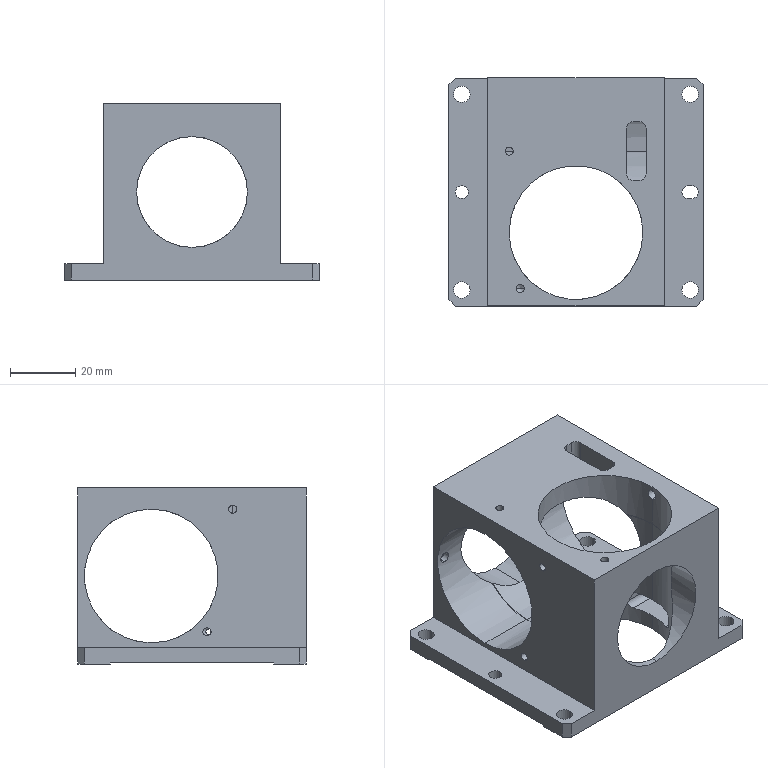Part | 1 solid | 83 faces | box 78 x 70 x 54 mm | volume 71307 mm3 | cylinder 45 | plane 33 | cone 5 | commonest cylinder face diameters 4 x13 2.5 x8 5 x8 3.3 x4 34 x4 41 x4